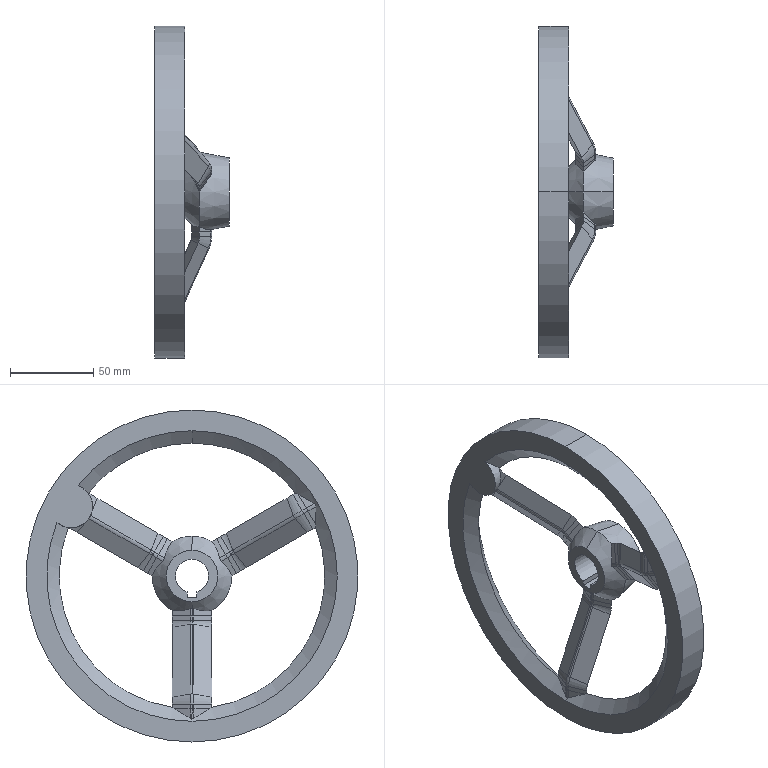Part | SolidWorks | features ICE 2, CirPattern 1, Revolution 1, Sweep 1 | 1 solid | 157 faces | box 45 x 200 x 200 mm | volume 211717 mm3 | plane 65 | cylinder 39 | cone 35 | torus 18 | commonest cylinder face diameters 6 x33 20 x2 26 x2 200 x2